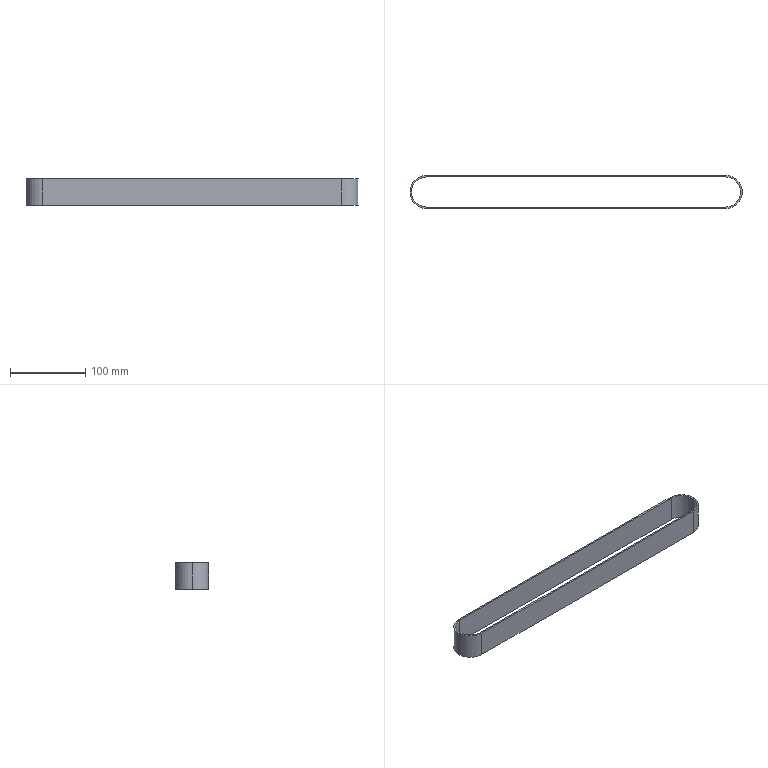Part | STEP file | Belt | 1 solid | 12 faces | box 442 x 44 x 35 mm | volume 64956 mm3 | cylinder 6 | plane 6 | commonest cylinder face diameters 40 x3 44 x3
STEP:
#1=CARTESIAN_POINT('',(0.,0.,0.));
#2=DIRECTION('',(0.,0.,1.));
#3=DIRECTION('',(1.,0.,0.));
#4=AXIS2_PLACEMENT_3D('',#1,#2,#3);
#5=CARTESIAN_POINT('',(-22.,0.,35.));
#6=VERTEX_POINT('',#5);
#7=CARTESIAN_POINT('',(0.,-22.,35.));
#8=VERTEX_POINT('',#7);
#9=CARTESIAN_POINT('',(0.,0.,35.));
#10=DIRECTION('',(0.,0.,1.));
#11=DIRECTION('',(-1.,0.,0.));
#12=AXIS2_PLACEMENT_3D('',#9,#10,#11);
#13=CIRCLE('',#12,22.);
#14=CARTESIAN_POINT('',(0.,0.,35.));
#15=DIRECTION('',(0.,0.,-1.));
#16=DIRECTION('',(-1.,0.,0.));
#17=AXIS2_PLACEMENT_3D('',#14,#15,#16);
#18=CYLINDRICAL_SURFACE('',#17,22.);
#19=CARTESIAN_POINT('',(6.283,0.));
#20=DIRECTION('',(-1.,0.));
#21=VECTOR('',#20,1.);
#22=LINE('',#19,#21);
#23=(GEOMETRIC_REPRESENTATION_CONTEXT(2)PARAMETRIC_REPRESENTATION_CONTEXT()REPRESENTATION_CONTEXT('',''));
#24=DEFINITIONAL_REPRESENTATION('',(#22),#23);
#25=PCURVE('',#18,#24);
#26=CARTESIAN_POINT('',(0.,0.,35.));
#27=DIRECTION('',(0.,0.,1.));
#28=DIRECTION('',(1.,0.,0.));
#29=AXIS2_PLACEMENT_3D('',#26,#27,#28);
#30=PLANE('',#29);
#31=CARTESIAN_POINT('',(0.,0.));
#32=DIRECTION('',(-1.,0.));
#33=AXIS2_PLACEMENT_2D('',#31,#32);
#34=CIRCLE('',#33,22.);
#35=(GEOMETRIC_REPRESENTATION_CONTEXT(2)PARAMETRIC_REPRESENTATION_CONTEXT()REPRESENTATION_CONTEXT('',''));
#36=DEFINITIONAL_REPRESENTATION('',(#34),#35);
#37=PCURVE('',#30,#36);
#38=SURFACE_CURVE('',#13,(#25,#37),.PCURVE_S1.);
#39=EDGE_CURVE('',#6,#8,#38,.T.);
#40=ORIENTED_EDGE('',*,*,#39,.F.);
#41=CARTESIAN_POINT('',(-22.,0.,0.));
#42=VERTEX_POINT('',#41);
#43=CARTESIAN_POINT('',(-22.,0.,35.));
#44=DIRECTION('',(0.,0.,-1.));
#45=VECTOR('',#44,1.);
#46=LINE('',#43,#45);
#47=CARTESIAN_POINT('',(6.283,0.));
#48=DIRECTION('',(0.,1.));
#49=VECTOR('',#48,1.);
#50=LINE('',#47,#49);
#51=(GEOMETRIC_REPRESENTATION_CONTEXT(2)PARAMETRIC_REPRESENTATION_CONTEXT()REPRESENTATION_CONTEXT('',''));
#52=DEFINITIONAL_REPRESENTATION('',(#50),#51);
#53=PCURVE('',#18,#52);
#54=CARTESIAN_POINT('',(0.,0.,35.));
#55=DIRECTION('',(0.,0.,-1.));
#56=DIRECTION('',(-1.,0.,0.));
#57=AXIS2_PLACEMENT_3D('',#54,#55,#56);
#58=CYLINDRICAL_SURFACE('',#57,22.);
#59=CARTESIAN_POINT('',(0.,0.));
#60=DIRECTION('',(0.,1.));
#61=VECTOR('',#60,1.);
#62=LINE('',#59,#61);
#63=(GEOMETRIC_REPRESENTATION_CONTEXT(2)PARAMETRIC_REPRESENTATION_CONTEXT()REPRESENTATION_CONTEXT('',''));
#64=DEFINITIONAL_REPRESENTATION('',(#62),#63);
#65=PCURVE('',#58,#64);
#66=SURFACE_CURVE('',#46,(#53,#65),.PCURVE_S1.);
#67=EDGE_CURVE('',#6,#42,#66,.T.);
#68=ORIENTED_EDGE('',*,*,#67,.T.);
#69=CARTESIAN_POINT('',(0.,-22.,0.));
#70=VERTEX_POINT('',#69);
#71=CARTESIAN_POINT('',(0.,0.,0.));
#72=DIRECTION('',(0.,0.,1.));
#73=DIRECTION('',(-1.,0.,0.));
#74=AXIS2_PLACEMENT_3D('',#71,#72,#73);
#75=CIRCLE('',#74,22.);
#76=CARTESIAN_POINT('',(6.283,35.));
#77=DIRECTION('',(-1.,0.));
#78=VECTOR('',#77,1.);
#79=LINE('',#76,#78);
#80=(GEOMETRIC_REPRESENTATION_CONTEXT(2)PARAMETRIC_REPRESENTATION_CONTEXT()REPRESENTATION_CONTEXT('',''));
#81=DEFINITIONAL_REPRESENTATION('',(#79),#80);
#82=PCURVE('',#18,#81);
#83=CARTESIAN_POINT('',(0.,0.,0.));
#84=DIRECTION('',(0.,0.,1.));
#85=DIRECTION('',(1.,0.,0.));
#86=AXIS2_PLACEMENT_3D('',#83,#84,#85);
#87=PLANE('',#86);
#88=CARTESIAN_POINT('',(0.,0.));
#89=DIRECTION('',(-1.,0.));
#90=AXIS2_PLACEMENT_2D('',#88,#89);
#91=CIRCLE('',#90,22.);
#92=(GEOMETRIC_REPRESENTATION_CONTEXT(2)PARAMETRIC_REPRESENTATION_CONTEXT()REPRESENTATION_CONTEXT('',''));
#93=DEFINITIONAL_REPRESENTATION('',(#91),#92);
#94=PCURVE('',#87,#93);
#95=SURFACE_CURVE('',#75,(#82,#94),.PCURVE_S1.);
#96=EDGE_CURVE('',#42,#70,#95,.T.);
#97=ORIENTED_EDGE('',*,*,#96,.T.);
#98=CARTESIAN_POINT('',(0.,-22.,35.));
#99=DIRECTION('',(0.,0.,1.));
#100=VECTOR('',#99,1.);
#101=LINE('',#98,#100);
#102=CARTESIAN_POINT('',(4.712,0.));
#103=DIRECTION('',(0.,-1.));
#104=VECTOR('',#103,1.);
#105=LINE('',#102,#104);
#106=(GEOMETRIC_REPRESENTATION_CONTEXT(2)PARAMETRIC_REPRESENTATION_CONTEXT()REPRESENTATION_CONTEXT('',''));
#107=DEFINITIONAL_REPRESENTATION('',(#105),#106);
#108=PCURVE('',#18,#107);
#109=CARTESIAN_POINT('',(0.,-22.,35.));
#110=DIRECTION('',(0.,1.,0.));
#111=DIRECTION('',(0.,0.,1.));
#112=AXIS2_PLACEMENT_3D('',#109,#110,#111);
#113=PLANE('',#112);
#114=CARTESIAN_POINT('',(0.,0.));
#115=DIRECTION('',(1.,0.));
#116=VECTOR('',#115,1.);
#117=LINE('',#114,#116);
#118=(GEOMETRIC_REPRESENTATION_CONTEXT(2)PARAMETRIC_REPRESENTATION_CONTEXT()REPRESENTATION_CONTEXT('',''));
#119=DEFINITIONAL_REPRESENTATION('',(#117),#118);
#120=PCURVE('',#113,#119);
#121=SURFACE_CURVE('',#101,(#108,#120),.PCURVE_S1.);
#122=EDGE_CURVE('',#70,#8,#121,.T.);
#123=ORIENTED_EDGE('',*,*,#122,.T.);
#124=EDGE_LOOP('',(#40,#68,#97,#123));
#125=FACE_BOUND('',#124,.T.);
#126=ADVANCED_FACE('',(#125),#18,.T.);
#127=CARTESIAN_POINT('',(0.,20.,35.));
#128=VERTEX_POINT('',#127);
#129=CARTESIAN_POINT('',(0.,20.,0.));
#130=VERTEX_POINT('',#129);
#131=CARTESIAN_POINT('',(0.,20.,35.));
#132=DIRECTION('',(0.,0.,-1.));
#133=VECTOR('',#132,1.);
#134=LINE('',#131,#133);
#135=CARTESIAN_POINT('',(0.,0.,35.));
#136=DIRECTION('',(0.,0.,-1.));
#137=DIRECTION('',(-1.,0.,0.));
#138=AXIS2_PLACEMENT_3D('',#135,#136,#137);
#139=CYLINDRICAL_SURFACE('',#138,20.);
#140=CARTESIAN_POINT('',(1.571,0.));
#141=DIRECTION('',(0.,1.));
#142=VECTOR('',#141,1.);
#143=LINE('',#140,#142);
#144=(GEOMETRIC_REPRESENTATION_CONTEXT(2)PARAMETRIC_REPRESENTATION_CONTEXT()REPRESENTATION_CONTEXT('',''));
#145=DEFINITIONAL_REPRESENTATION('',(#143),#144);
#146=PCURVE('',#139,#145);
#147=CARTESIAN_POINT('',(0.,20.,35.));
#148=DIRECTION('',(0.,-1.,0.));
#149=DIRECTION('',(0.,0.,-1.));
#150=AXIS2_PLACEMENT_3D('',#147,#148,#149);
#151=PLANE('',#150);
#152=CARTESIAN_POINT('',(0.,0.));
#153=DIRECTION('',(1.,0.));
#154=VECTOR('',#153,1.);
#155=LINE('',#152,#154);
#156=(GEOMETRIC_REPRESENTATION_CONTEXT(2)PARAMETRIC_REPRESENTATION_CONTEXT()REPRESENTATION_CONTEXT('',''));
#157=DEFINITIONAL_REPRESENTATION('',(#155),#156);
#158=PCURVE('',#151,#157);
#159=SURFACE_CURVE('',#134,(#146,#158),.PCURVE_S1.);
#160=EDGE_CURVE('',#128,#130,#159,.T.);
#161=ORIENTED_EDGE('',*,*,#160,.T.);
#162=CARTESIAN_POINT('',(-20.,0.,0.));
#163=VERTEX_POINT('',#162);
#164=CARTESIAN_POINT('',(0.,0.,0.));
#165=DIRECTION('',(0.,0.,-1.));
#166=DIRECTION('',(-1.,0.,0.));
#167=AXIS2_PLACEMENT_3D('',#164,#165,#166);
#168=CIRCLE('',#167,20.);
#169=CARTESIAN_POINT('',(0.,35.));
#170=DIRECTION('',(1.,0.));
#171=VECTOR('',#170,1.);
#172=LINE('',#169,#171);
#173=(GEOMETRIC_REPRESENTATION_CONTEXT(2)PARAMETRIC_REPRESENTATION_CONTEXT()REPRESENTATION_CONTEXT('',''));
#174=DEFINITIONAL_REPRESENTATION('',(#172),#173);
#175=PCURVE('',#139,#174);
#176=CARTESIAN_POINT('',(-20.,0.));
#177=CARTESIAN_POINT('',(-20.,34.641));
#178=CARTESIAN_POINT('',(10.,17.321));
#179=CARTESIAN_POINT('',(40.,0.));
#180=CARTESIAN_POINT('',(10.,-17.321));
#181=CARTESIAN_POINT('',(-20.,-34.641));
#182=CARTESIAN_POINT('',(-20.,0.));
#183=(BOUNDED_CURVE()B_SPLINE_CURVE(2,(#176,#177,#178,#179,#180,#181,#182),.UNSPECIFIED.,.T.,.F.)B_SPLINE_CURVE_WITH_KNOTS((1,2,2,2,2,1),(-2.094,0.,2.094,4.189,6.283,8.378),.UNSPECIFIED.)CURVE()GEOMETRIC_REPRESENTATION_ITEM()RATIONAL_B_SPLINE_CURVE((1.,0.5,1.,0.5,1.,0.5,1.))REPRESENTATION_ITEM(''));
#184=(GEOMETRIC_REPRESENTATION_CONTEXT(2)PARAMETRIC_REPRESENTATION_CONTEXT()REPRESENTATION_CONTEXT('',''));
#185=DEFINITIONAL_REPRESENTATION('',(#183),#184);
#186=PCURVE('',#87,#185);
#187=SURFACE_CURVE('',#168,(#175,#186),.PCURVE_S1.);
#188=EDGE_CURVE('',#163,#130,#187,.T.);
#189=ORIENTED_EDGE('',*,*,#188,.F.);
#190=CARTESIAN_POINT('',(-20.,0.,35.));
#191=VERTEX_POINT('',#190);
#192=CARTESIAN_POINT('',(-20.,0.,35.));
#193=DIRECTION('',(0.,0.,-1.));
#194=VECTOR('',#193,1.);
#195=LINE('',#192,#194);
#196=CARTESIAN_POINT('',(0.,0.));
#197=DIRECTION('',(0.,1.));
#198=VECTOR('',#197,1.);
#199=LINE('',#196,#198);
#200=(GEOMETRIC_REPRESENTATION_CONTEXT(2)PARAMETRIC_REPRESENTATION_CONTEXT()REPRESENTATION_CONTEXT('',''));
#201=DEFINITIONAL_REPRESENTATION('',(#199),#200);
#202=PCURVE('',#139,#201);
#203=CARTESIAN_POINT('',(0.,0.,35.));
#204=DIRECTION('',(0.,0.,-1.));
#205=DIRECTION('',(-1.,0.,0.));
#206=AXIS2_PLACEMENT_3D('',#203,#204,#205);
#207=CYLINDRICAL_SURFACE('',#206,20.);
#208=CARTESIAN_POINT('',(6.283,0.));
#209=DIRECTION('',(0.,1.));
#210=VECTOR('',#209,1.);
#211=LINE('',#208,#210);
#212=(GEOMETRIC_REPRESENTATION_CONTEXT(2)PARAMETRIC_REPRESENTATION_CONTEXT()REPRESENTATION_CONTEXT('',''));
#213=DEFINITIONAL_REPRESENTATION('',(#211),#212);
#214=PCURVE('',#207,#213);
#215=SURFACE_CURVE('',#195,(#202,#214),.PCURVE_S1.);
#216=EDGE_CURVE('',#191,#163,#215,.T.);
#217=ORIENTED_EDGE('',*,*,#216,.F.);
#218=CARTESIAN_POINT('',(0.,0.,35.));
#219=DIRECTION('',(0.,0.,-1.));
#220=DIRECTION('',(-1.,0.,0.));
#221=AXIS2_PLACEMENT_3D('',#218,#219,#220);
#222=CIRCLE('',#221,20.);
#223=CARTESIAN_POINT('',(0.,0.));
#224=DIRECTION('',(1.,0.));
#225=VECTOR('',#224,1.);
#226=LINE('',#223,#225);
#227=(GEOMETRIC_REPRESENTATION_CONTEXT(2)PARAMETRIC_REPRESENTATION_CONTEXT()REPRESENTATION_CONTEXT('',''));
#228=DEFINITIONAL_REPRESENTATION('',(#226),#227);
#229=PCURVE('',#139,#228);
#230=CARTESIAN_POINT('',(-20.,0.));
#231=CARTESIAN_POINT('',(-20.,34.641));
#232=CARTESIAN_POINT('',(10.,17.321));
#233=CARTESIAN_POINT('',(40.,0.));
#234=CARTESIAN_POINT('',(10.,-17.321));
#235=CARTESIAN_POINT('',(-20.,-34.641));
#236=CARTESIAN_POINT('',(-20.,0.));
#237=(BOUNDED_CURVE()B_SPLINE_CURVE(2,(#230,#231,#232,#233,#234,#235,#236),.UNSPECIFIED.,.T.,.F.)B_SPLINE_CURVE_WITH_KNOTS((1,2,2,2,2,1),(-2.094,0.,2.094,4.189,6.283,8.378),.UNSPECIFIED.)CURVE()GEOMETRIC_REPRESENTATION_ITEM()RATIONAL_B_SPLINE_CURVE((1.,0.5,1.,0.5,1.,0.5,1.))REPRESENTATION_ITEM(''));
#238=(GEOMETRIC_REPRESENTATION_CONTEXT(2)PARAMETRIC_REPRESENTATION_CONTEXT()REPRESENTATION_CONTEXT('',''));
#239=DEFINITIONAL_REPRESENTATION('',(#237),#238);
#240=PCURVE('',#30,#239);
#241=SURFACE_CURVE('',#222,(#229,#240),.PCURVE_S1.);
#242=EDGE_CURVE('',#191,#128,#241,.T.);
#243=ORIENTED_EDGE('',*,*,#242,.T.);
#244=EDGE_LOOP('',(#161,#189,#217,#243));
#245=FACE_BOUND('',#244,.F.);
#246=ADVANCED_FACE('',(#245),#139,.F.);
#247=CARTESIAN_POINT('',(398.,-22.,35.));
#248=VERTEX_POINT('',#247);
#249=CARTESIAN_POINT('',(398.,-22.,0.));
#250=VERTEX_POINT('',#249);
#251=CARTESIAN_POINT('',(398.,-22.,35.));
#252=DIRECTION('',(0.,0.,-1.));
#253=VECTOR('',#252,1.);
#254=LINE('',#251,#253);
#255=CARTESIAN_POINT('',(0.,398.));
#256=DIRECTION('',(-1.,0.));
#257=VECTOR('',#256,1.);
#258=LINE('',#255,#257);
#259=(GEOMETRIC_REPRESENTATION_CONTEXT(2)PARAMETRIC_REPRESENTATION_CONTEXT()REPRESENTATION_CONTEXT('',''));
#260=DEFINITIONAL_REPRESENTATION('',(#258),#259);
#261=PCURVE('',#113,#260);
#262=CARTESIAN_POINT('',(398.,0.,35.));
#263=DIRECTION('',(0.,0.,-1.));
#264=DIRECTION('',(-1.,0.,0.));
#265=AXIS2_PLACEMENT_3D('',#262,#263,#264);
#266=CYLINDRICAL_SURFACE('',#265,22.);
#267=CARTESIAN_POINT('',(4.712,0.));
#268=DIRECTION('',(0.,1.));
#269=VECTOR('',#268,1.);
#270=LINE('',#267,#269);
#271=(GEOMETRIC_REPRESENTATION_CONTEXT(2)PARAMETRIC_REPRESENTATION_CONTEXT()REPRESENTATION_CONTEXT('',''));
#272=DEFINITIONAL_REPRESENTATION('',(#270),#271);
#273=PCURVE('',#266,#272);
#274=SURFACE_CURVE('',#254,(#261,#273),.PCURVE_S1.);
#275=EDGE_CURVE('',#248,#250,#274,.T.);
#276=ORIENTED_EDGE('',*,*,#275,.F.);
#277=CARTESIAN_POINT('',(0.,-22.,35.));
#278=DIRECTION('',(1.,0.,0.));
#279=VECTOR('',#278,1.);
#280=LINE('',#277,#279);
#281=CARTESIAN_POINT('',(0.,0.));
#282=DIRECTION('',(0.,1.));
#283=VECTOR('',#282,1.);
#284=LINE('',#281,#283);
#285=(GEOMETRIC_REPRESENTATION_CONTEXT(2)PARAMETRIC_REPRESENTATION_CONTEXT()REPRESENTATION_CONTEXT('',''));
#286=DEFINITIONAL_REPRESENTATION('',(#284),#285);
#287=PCURVE('',#113,#286);
#288=CARTESIAN_POINT('',(0.,-22.));
#289=DIRECTION('',(1.,0.));
#290=VECTOR('',#289,1.);
#291=LINE('',#288,#290);
#292=(GEOMETRIC_REPRESENTATION_CONTEXT(2)PARAMETRIC_REPRESENTATION_CONTEXT()REPRESENTATION_CONTEXT('',''));
#293=DEFINITIONAL_REPRESENTATION('',(#291),#292);
#294=PCURVE('',#30,#293);
#295=SURFACE_CURVE('',#280,(#287,#294),.PCURVE_S1.);
#296=EDGE_CURVE('',#8,#248,#295,.T.);
#297=ORIENTED_EDGE('',*,*,#296,.F.);
#298=ORIENTED_EDGE('',*,*,#122,.F.);
#299=CARTESIAN_POINT('',(0.,-22.,0.));
#300=DIRECTION('',(-1.,0.,0.));
#301=VECTOR('',#300,1.);
#302=LINE('',#299,#301);
#303=CARTESIAN_POINT('',(-35.,0.));
#304=DIRECTION('',(0.,-1.));
#305=VECTOR('',#304,1.);
#306=LINE('',#303,#305);
#307=(GEOMETRIC_REPRESENTATION_CONTEXT(2)PARAMETRIC_REPRESENTATION_CONTEXT()REPRESENTATION_CONTEXT('',''));
#308=DEFINITIONAL_REPRESENTATION('',(#306),#307);
#309=PCURVE('',#113,#308);
#310=CARTESIAN_POINT('',(0.,-22.));
#311=DIRECTION('',(-1.,0.));
#312=VECTOR('',#311,1.);
#313=LINE('',#310,#312);
#314=(GEOMETRIC_REPRESENTATION_CONTEXT(2)PARAMETRIC_REPRESENTATION_CONTEXT()REPRESENTATION_CONTEXT('',''));
#315=DEFINITIONAL_REPRESENTATION('',(#313),#314);
#316=PCURVE('',#87,#315);
#317=SURFACE_CURVE('',#302,(#309,#316),.PCURVE_S1.);
#318=EDGE_CURVE('',#250,#70,#317,.T.);
#319=ORIENTED_EDGE('',*,*,#318,.F.);
#320=EDGE_LOOP('',(#276,#297,#298,#319));
#321=FACE_BOUND('',#320,.T.);
#322=ADVANCED_FACE('',(#321),#113,.F.);
#323=CARTESIAN_POINT('',(0.,-20.,0.));
#324=VERTEX_POINT('',#323);
#325=CARTESIAN_POINT('',(0.,0.,0.));
#326=DIRECTION('',(0.,0.,-1.));
#327=DIRECTION('',(-1.,0.,0.));
#328=AXIS2_PLACEMENT_3D('',#325,#326,#327);
#329=CIRCLE('',#328,20.);
#330=CARTESIAN_POINT('',(-20.,0.));
#331=CARTESIAN_POINT('',(-20.,34.641));
#332=CARTESIAN_POINT('',(10.,17.321));
#333=CARTESIAN_POINT('',(40.,0.));
#334=CARTESIAN_POINT('',(10.,-17.321));
#335=CARTESIAN_POINT('',(-20.,-34.641));
#336=CARTESIAN_POINT('',(-20.,0.));
#337=(BOUNDED_CURVE()B_SPLINE_CURVE(2,(#330,#331,#332,#333,#334,#335,#336),.UNSPECIFIED.,.T.,.F.)B_SPLINE_CURVE_WITH_KNOTS((1,2,2,2,2,1),(-2.094,0.,2.094,4.189,6.283,8.378),.UNSPECIFIED.)CURVE()GEOMETRIC_REPRESENTATION_ITEM()RATIONAL_B_SPLINE_CURVE((1.,0.5,1.,0.5,1.,0.5,1.))REPRESENTATION_ITEM(''));
#338=(GEOMETRIC_REPRESENTATION_CONTEXT(2)PARAMETRIC_REPRESENTATION_CONTEXT()REPRESENTATION_CONTEXT('',''));
#339=DEFINITIONAL_REPRESENTATION('',(#337),#338);
#340=PCURVE('',#87,#339);
#341=CARTESIAN_POINT('',(0.,35.));
#342=DIRECTION('',(1.,0.));
#343=VECTOR('',#342,1.);
#344=LINE('',#341,#343);
#345=(GEOMETRIC_REPRESENTATION_CONTEXT(2)PARAMETRIC_REPRESENTATION_CONTEXT()REPRESENTATION_CONTEXT('',''));
#346=DEFINITIONAL_REPRESENTATION('',(#344),#345);
#347=PCURVE('',#207,#346);
#348=SURFACE_CURVE('',#329,(#340,#347),.PCURVE_S1.);
#349=EDGE_CURVE('',#324,#163,#348,.T.);
#350=ORIENTED_EDGE('',*,*,#349,.F.);
#351=CARTESIAN_POINT('',(398.,-20.,0.));
#352=VERTEX_POINT('',#351);
#353=CARTESIAN_POINT('',(0.,-20.,0.));
#354=DIRECTION('',(-1.,0.,0.));
#355=VECTOR('',#354,1.);
#356=LINE('',#353,#355);
#357=CARTESIAN_POINT('',(0.,-20.));
#358=DIRECTION('',(-1.,0.));
#359=VECTOR('',#358,1.);
#360=LINE('',#357,#359);
#361=(GEOMETRIC_REPRESENTATION_CONTEXT(2)PARAMETRIC_REPRESENTATION_CONTEXT()REPRESENTATION_CONTEXT('',''));
#362=DEFINITIONAL_REPRESENTATION('',(#360),#361);
#363=PCURVE('',#87,#362);
#364=CARTESIAN_POINT('',(0.,-20.,35.));
#365=DIRECTION('',(0.,1.,0.));
#366=DIRECTION('',(0.,0.,1.));
#367=AXIS2_PLACEMENT_3D('',#364,#365,#366);
#368=PLANE('',#367);
#369=CARTESIAN_POINT('',(-35.,0.));
#370=DIRECTION('',(0.,-1.));
#371=VECTOR('',#370,1.);
#372=LINE('',#369,#371);
#373=(GEOMETRIC_REPRESENTATION_CONTEXT(2)PARAMETRIC_REPRESENTATION_CONTEXT()REPRESENTATION_CONTEXT('',''));
#374=DEFINITIONAL_REPRESENTATION('',(#372),#373);
#375=PCURVE('',#368,#374);
#376=SURFACE_CURVE('',#356,(#363,#375),.PCURVE_S1.);
#377=EDGE_CURVE('',#352,#324,#376,.T.);
#378=ORIENTED_EDGE('',*,*,#377,.F.);
#379=CARTESIAN_POINT('',(398.,20.,0.));
#380=VERTEX_POINT('',#379);
#381=CARTESIAN_POINT('',(398.,0.,0.));
#382=DIRECTION('',(0.,0.,-1.));
#383=DIRECTION('',(-1.,0.,0.));
#384=AXIS2_PLACEMENT_3D('',#381,#382,#383);
#385=CIRCLE('',#384,20.);
#386=CARTESIAN_POINT('',(378.,0.));
#387=CARTESIAN_POINT('',(378.,34.641));
#388=CARTESIAN_POINT('',(408.,17.321));
#389=CARTESIAN_POINT('',(438.,0.));
#390=CARTESIAN_POINT('',(408.,-17.321));
#391=CARTESIAN_POINT('',(378.,-34.641));
#392=CARTESIAN_POINT('',(378.,0.));
#393=(BOUNDED_CURVE()B_SPLINE_CURVE(2,(#386,#387,#388,#389,#390,#391,#392),.UNSPECIFIED.,.T.,.F.)B_SPLINE_CURVE_WITH_KNOTS((1,2,2,2,2,1),(-2.094,0.,2.094,4.189,6.283,8.378),.UNSPECIFIED.)CURVE()GEOMETRIC_REPRESENTATION_ITEM()RATIONAL_B_SPLINE_CURVE((1.,0.5,1.,0.5,1.,0.5,1.))REPRESENTATION_ITEM(''));
#394=(GEOMETRIC_REPRESENTATION_CONTEXT(2)PARAMETRIC_REPRESENTATION_CONTEXT()REPRESENTATION_CONTEXT('',''));
#395=DEFINITIONAL_REPRESENTATION('',(#393),#394);
#396=PCURVE('',#87,#395);
#397=CARTESIAN_POINT('',(398.,0.,35.));
#398=DIRECTION('',(0.,0.,-1.));
#399=DIRECTION('',(-1.,0.,0.));
#400=AXIS2_PLACEMENT_3D('',#397,#398,#399);
#401=CYLINDRICAL_SURFACE('',#400,20.);
#402=CARTESIAN_POINT('',(0.,35.));
#403=DIRECTION('',(1.,0.));
#404=VECTOR('',#403,1.);
#405=LINE('',#402,#404);
#406=(GEOMETRIC_REPRESENTATION_CONTEXT(2)PARAMETRIC_REPRESENTATION_CONTEXT()REPRESENTATION_CONTEXT('',''));
#407=DEFINITIONAL_REPRESENTATION('',(#405),#406);
#408=PCURVE('',#401,#407);
#409=SURFACE_CURVE('',#385,(#396,#408),.PCURVE_S1.);
#410=EDGE_CURVE('',#380,#352,#409,.T.);
#411=ORIENTED_EDGE('',*,*,#410,.F.);
#412=CARTESIAN_POINT('',(0.,20.,0.));
#413=DIRECTION('',(1.,0.,0.));
#414=VECTOR('',#413,1.);
#415=LINE('',#412,#414);
#416=CARTESIAN_POINT('',(0.,20.));
#417=DIRECTION('',(1.,0.));
#418=VECTOR('',#417,1.);
#419=LINE('',#416,#418);
#420=(GEOMETRIC_REPRESENTATION_CONTEXT(2)PARAMETRIC_REPRESENTATION_CONTEXT()REPRESENTATION_CONTEXT('',''));
#421=DEFINITIONAL_REPRESENTATION('',(#419),#420);
#422=PCURVE('',#87,#421);
#423=CARTESIAN_POINT('',(35.,0.));
#424=DIRECTION('',(0.,1.));
#425=VECTOR('',#424,1.);
#426=LINE('',#423,#425);
#427=(GEOMETRIC_REPRESENTATION_CONTEXT(2)PARAMETRIC_REPRESENTATION_CONTEXT()REPRESENTATION_CONTEXT('',''));
#428=DEFINITIONAL_REPRESENTATION('',(#426),#427);
#429=PCURVE('',#151,#428);
#430=SURFACE_CURVE('',#415,(#422,#429),.PCURVE_S1.);
#431=EDGE_CURVE('',#130,#380,#430,.T.);
#432=ORIENTED_EDGE('',*,*,#431,.F.);
#433=ORIENTED_EDGE('',*,*,#188,.F.);
#434=EDGE_LOOP('',(#350,#378,#411,#432,#433));
#435=FACE_BOUND('',#434,.T.);
#436=CARTESIAN_POINT('',(398.,22.,0.));
#437=VERTEX_POINT('',#436);
#438=CARTESIAN_POINT('',(0.,22.,0.));
#439=VERTEX_POINT('',#438);
#440=CARTESIAN_POINT('',(0.,22.,0.));
#441=DIRECTION('',(-1.,0.,0.));
#442=VECTOR('',#441,1.);
#443=LINE('',#440,#442);
#444=CARTESIAN_POINT('',(0.,22.));
#445=DIRECTION('',(-1.,0.));
#446=VECTOR('',#445,1.);
#447=LINE('',#444,#446);
#448=(GEOMETRIC_REPRESENTATION_CONTEXT(2)PARAMETRIC_REPRESENTATION_CONTEXT()REPRESENTATION_CONTEXT('',''));
#449=DEFINITIONAL_REPRESENTATION('',(#447),#448);
#450=PCURVE('',#87,#449);
#451=CARTESIAN_POINT('',(0.,22.,35.));
#452=DIRECTION('',(0.,-1.,0.));
#453=DIRECTION('',(0.,0.,-1.));
#454=AXIS2_PLACEMENT_3D('',#451,#452,#453);
#455=PLANE('',#454);
#456=CARTESIAN_POINT('',(35.,0.));
#457=DIRECTION('',(0.,-1.));
#458=VECTOR('',#457,1.);
#459=LINE('',#456,#458);
#460=(GEOMETRIC_REPRESENTATION_CONTEXT(2)PARAMETRIC_REPRESENTATION_CONTEXT()REPRESENTATION_CONTEXT('',''));
#461=DEFINITIONAL_REPRESENTATION('',(#459),#460);
#462=PCURVE('',#455,#461);
#463=SURFACE_CURVE('',#443,(#450,#462),.PCURVE_S1.);
#464=EDGE_CURVE('',#437,#439,#463,.T.);
#465=ORIENTED_EDGE('',*,*,#464,.F.);
#466=CARTESIAN_POINT('',(398.,0.,0.));
#467=DIRECTION('',(0.,0.,1.));
#468=DIRECTION('',(-1.,0.,0.));
#469=AXIS2_PLACEMENT_3D('',#466,#467,#468);
#470=CIRCLE('',#469,22.);
#471=CARTESIAN_POINT('',(398.,0.));
#472=DIRECTION('',(-1.,0.));
#473=AXIS2_PLACEMENT_2D('',#471,#472);
#474=CIRCLE('',#473,22.);
#475=(GEOMETRIC_REPRESENTATION_CONTEXT(2)PARAMETRIC_REPRESENTATION_CONTEXT()REPRESENTATION_CONTEXT('',''));
#476=DEFINITIONAL_REPRESENTATION('',(#474),#475);
#477=PCURVE('',#87,#476);
#478=CARTESIAN_POINT('',(6.283,35.));
#479=DIRECTION('',(-1.,0.));
#480=VECTOR('',#479,1.);
#481=LINE('',#478,#480);
#482=(GEOMETRIC_REPRESENTATION_CONTEXT(2)PARAMETRIC_REPRESENTATION_CONTEXT()REPRESENTATION_CONTEXT('',''));
#483=DEFINITIONAL_REPRESENTATION('',(#481),#482);
#484=PCURVE('',#266,#483);
#485=SURFACE_CURVE('',#470,(#477,#484),.PCURVE_S1.);
#486=EDGE_CURVE('',#250,#437,#485,.T.);
#487=ORIENTED_EDGE('',*,*,#486,.F.);
#488=ORIENTED_EDGE('',*,*,#318,.T.);
#489=ORIENTED_EDGE('',*,*,#96,.F.);
#490=CARTESIAN_POINT('',(0.,0.,0.));
#491=DIRECTION('',(0.,0.,1.));
#492=DIRECTION('',(-1.,0.,0.));
#493=AXIS2_PLACEMENT_3D('',#490,#491,#492);
#494=CIRCLE('',#493,22.);
#495=CARTESIAN_POINT('',(0.,0.));
#496=DIRECTION('',(-1.,0.));
#497=AXIS2_PLACEMENT_2D('',#495,#496);
#498=CIRCLE('',#497,22.);
#499=(GEOMETRIC_REPRESENTATION_CONTEXT(2)PARAMETRIC_REPRESENTATION_CONTEXT()REPRESENTATION_CONTEXT('',''));
#500=DEFINITIONAL_REPRESENTATION('',(#498),#499);
#501=PCURVE('',#87,#500);
#502=CARTESIAN_POINT('',(6.283,35.));
#503=DIRECTION('',(-1.,0.));
#504=VECTOR('',#503,1.);
#505=LINE('',#502,#504);
#506=(GEOMETRIC_REPRESENTATION_CONTEXT(2)PARAMETRIC_REPRESENTATION_CONTEXT()REPRESENTATION_CONTEXT('',''));
#507=DEFINITIONAL_REPRESENTATION('',(#505),#506);
#508=PCURVE('',#58,#507);
#509=SURFACE_CURVE('',#494,(#501,#508),.PCURVE_S1.);
#510=EDGE_CURVE('',#439,#42,#509,.T.);
#511=ORIENTED_EDGE('',*,*,#510,.F.);
#512=EDGE_LOOP('',(#465,#487,#488,#489,#511));
#513=FACE_BOUND('',#512,.T.);
#514=ADVANCED_FACE('',(#435,#513),#87,.F.);
#515=CARTESIAN_POINT('',(398.,22.,35.));
#516=VERTEX_POINT('',#515);
#517=CARTESIAN_POINT('',(398.,0.,35.));
#518=DIRECTION('',(0.,0.,-1.));
#519=DIRECTION('',(-1.,0.,0.));
#520=AXIS2_PLACEMENT_3D('',#517,#518,#519);
#521=CIRCLE('',#520,22.);
#522=CARTESIAN_POINT('',(0.,0.));
#523=DIRECTION('',(1.,0.));
#524=VECTOR('',#523,1.);
#525=LINE('',#522,#524);
#526=(GEOMETRIC_REPRESENTATION_CONTEXT(2)PARAMETRIC_REPRESENTATION_CONTEXT()REPRESENTATION_CONTEXT('',''));
#527=DEFINITIONAL_REPRESENTATION('',(#525),#526);
#528=PCURVE('',#266,#527);
#529=CARTESIAN_POINT('',(376.,0.));
#530=CARTESIAN_POINT('',(376.,38.105));
#531=CARTESIAN_POINT('',(409.,19.053));
#532=CARTESIAN_POINT('',(442.,0.));
#533=CARTESIAN_POINT('',(409.,-19.053));
#534=CARTESIAN_POINT('',(376.,-38.105));
#535=CARTESIAN_POINT('',(376.,0.));
#536=(BOUNDED_CURVE()B_SPLINE_CURVE(2,(#529,#530,#531,#532,#533,#534,#535),.UNSPECIFIED.,.T.,.F.)B_SPLINE_CURVE_WITH_KNOTS((1,2,2,2,2,1),(-2.094,0.,2.094,4.189,6.283,8.378),.UNSPECIFIED.)CURVE()GEOMETRIC_REPRESENTATION_ITEM()RATIONAL_B_SPLINE_CURVE((1.,0.5,1.,0.5,1.,0.5,1.))REPRESENTATION_ITEM(''));
#537=(GEOMETRIC_REPRESENTATION_CONTEXT(2)PARAMETRIC_REPRESENTATION_CONTEXT()REPRESENTATION_CONTEXT('',''));
#538=DEFINITIONAL_REPRESENTATION('',(#536),#537);
#539=PCURVE('',#30,#538);
#540=SURFACE_CURVE('',#521,(#528,#539),.PCURVE_S1.);
#541=EDGE_CURVE('',#516,#248,#540,.T.);
#542=ORIENTED_EDGE('',*,*,#541,.T.);
#543=ORIENTED_EDGE('',*,*,#275,.T.);
#544=ORIENTED_EDGE('',*,*,#486,.T.);
#545=CARTESIAN_POINT('',(398.,22.,35.));
#546=DIRECTION('',(0.,0.,1.));
#547=VECTOR('',#546,1.);
#548=LINE('',#545,#547);
#549=CARTESIAN_POINT('',(1.571,0.));
#550=DIRECTION('',(0.,-1.));
#551=VECTOR('',#550,1.);
#552=LINE('',#549,#551);
#553=(GEOMETRIC_REPRESENTATION_CONTEXT(2)PARAMETRIC_REPRESENTATION_CONTEXT()REPRESENTATION_CONTEXT('',''));
#554=DEFINITIONAL_REPRESENTATION('',(#552),#553);
#555=PCURVE('',#266,#554);
#556=CARTESIAN_POINT('',(0.,398.));
#557=DIRECTION('',(-1.,0.));
#558=VECTOR('',#557,1.);
#559=LINE('',#556,#558);
#560=(GEOMETRIC_REPRESENTATION_CONTEXT(2)PARAMETRIC_REPRESENTATION_CONTEXT()REPRESENTATION_CONTEXT('',''));
#561=DEFINITIONAL_REPRESENTATION('',(#559),#560);
#562=PCURVE('',#455,#561);
#563=SURFACE_CURVE('',#548,(#555,#562),.PCURVE_S1.);
#564=EDGE_CURVE('',#437,#516,#563,.T.);
#565=ORIENTED_EDGE('',*,*,#564,.T.);
#566=EDGE_LOOP('',(#542,#543,#544,#565));
#567=FACE_BOUND('',#566,.T.);
#568=ADVANCED_FACE('',(#567),#266,.T.);
#569=CARTESIAN_POINT('',(398.,20.,35.));
#570=VERTEX_POINT('',#569);
#571=CARTESIAN_POINT('',(0.,20.,35.));
#572=DIRECTION('',(1.,0.,0.));
#573=VECTOR('',#572,1.);
#574=LINE('',#571,#573);
#575=CARTESIAN_POINT('',(0.,20.));
#576=DIRECTION('',(1.,0.));
#577=VECTOR('',#576,1.);
#578=LINE('',#575,#577);
#579=(GEOMETRIC_REPRESENTATION_CONTEXT(2)PARAMETRIC_REPRESENTATION_CONTEXT()REPRESENTATION_CONTEXT('',''));
#580=DEFINITIONAL_REPRESENTATION('',(#578),#579);
#581=PCURVE('',#30,#580);
#582=CARTESIAN_POINT('',(0.,0.));
#583=DIRECTION('',(0.,1.));
#584=VECTOR('',#583,1.);
#585=LINE('',#582,#584);
#586=(GEOMETRIC_REPRESENTATION_CONTEXT(2)PARAMETRIC_REPRESENTATION_CONTEXT()REPRESENTATION_CONTEXT('',''));
#587=DEFINITIONAL_REPRESENTATION('',(#585),#586);
#588=PCURVE('',#151,#587);
#589=SURFACE_CURVE('',#574,(#581,#588),.PCURVE_S1.);
#590=EDGE_CURVE('',#128,#570,#589,.T.);
#591=ORIENTED_EDGE('',*,*,#590,.T.);
#592=CARTESIAN_POINT('',(398.,-20.,35.));
#593=VERTEX_POINT('',#592);
#594=CARTESIAN_POINT('',(398.,0.,35.));
#595=DIRECTION('',(0.,0.,-1.));
#596=DIRECTION('',(-1.,0.,0.));
#597=AXIS2_PLACEMENT_3D('',#594,#595,#596);
#598=CIRCLE('',#597,20.);
#599=CARTESIAN_POINT('',(378.,0.));
#600=CARTESIAN_POINT('',(378.,34.641));
#601=CARTESIAN_POINT('',(408.,17.321));
#602=CARTESIAN_POINT('',(438.,0.));
#603=CARTESIAN_POINT('',(408.,-17.321));
#604=CARTESIAN_POINT('',(378.,-34.641));
#605=CARTESIAN_POINT('',(378.,0.));
#606=(BOUNDED_CURVE()B_SPLINE_CURVE(2,(#599,#600,#601,#602,#603,#604,#605),.UNSPECIFIED.,.T.,.F.)B_SPLINE_CURVE_WITH_KNOTS((1,2,2,2,2,1),(-2.094,0.,2.094,4.189,6.283,8.378),.UNSPECIFIED.)CURVE()GEOMETRIC_REPRESENTATION_ITEM()RATIONAL_B_SPLINE_CURVE((1.,0.5,1.,0.5,1.,0.5,1.))REPRESENTATION_ITEM(''));
#607=(GEOMETRIC_REPRESENTATION_CONTEXT(2)PARAMETRIC_REPRESENTATION_CONTEXT()REPRESENTATION_CONTEXT('',''));
#608=DEFINITIONAL_REPRESENTATION('',(#606),#607);
#609=PCURVE('',#30,#608);
#610=CARTESIAN_POINT('',(0.,0.));
#611=DIRECTION('',(1.,0.));
#612=VECTOR('',#611,1.);
#613=LINE('',#610,#612);
#614=(GEOMETRIC_REPRESENTATION_CONTEXT(2)PARAMETRIC_REPRESENTATION_CONTEXT()REPRESENTATION_CONTEXT('',''));
#615=DEFINITIONAL_REPRESENTATION('',(#613),#614);
#616=PCURVE('',#401,#615);
#617=SURFACE_CURVE('',#598,(#609,#616),.PCURVE_S1.);
#618=EDGE_CURVE('',#570,#593,#617,.T.);
#619=ORIENTED_EDGE('',*,*,#618,.T.);
#620=CARTESIAN_POINT('',(0.,-20.,35.));
#621=VERTEX_POINT('',#620);
#622=CARTESIAN_POINT('',(0.,-20.,35.));
#623=DIRECTION('',(-1.,0.,0.));
#624=VECTOR('',#623,1.);
#625=LINE('',#622,#624);
#626=CARTESIAN_POINT('',(0.,-20.));
#627=DIRECTION('',(-1.,0.));
#628=VECTOR('',#627,1.);
#629=LINE('',#626,#628);
#630=(GEOMETRIC_REPRESENTATION_CONTEXT(2)PARAMETRIC_REPRESENTATION_CONTEXT()REPRESENTATION_CONTEXT('',''));
#631=DEFINITIONAL_REPRESENTATION('',(#629),#630);
#632=PCURVE('',#30,#631);
#633=CARTESIAN_POINT('',(0.,0.));
#634=DIRECTION('',(0.,-1.));
#635=VECTOR('',#634,1.);
#636=LINE('',#633,#635);
#637=(GEOMETRIC_REPRESENTATION_CONTEXT(2)PARAMETRIC_REPRESENTATION_CONTEXT()REPRESENTATION_CONTEXT('',''));
#638=DEFINITIONAL_REPRESENTATION('',(#636),#637);
#639=PCURVE('',#368,#638);
#640=SURFACE_CURVE('',#625,(#632,#639),.PCURVE_S1.);
#641=EDGE_CURVE('',#593,#621,#640,.T.);
#642=ORIENTED_EDGE('',*,*,#641,.T.);
#643=CARTESIAN_POINT('',(0.,0.,35.));
#644=DIRECTION('',(0.,0.,-1.));
#645=DIRECTION('',(-1.,0.,0.));
#646=AXIS2_PLACEMENT_3D('',#643,#644,#645);
#647=CIRCLE('',#646,20.);
#648=CARTESIAN_POINT('',(-20.,0.));
#649=CARTESIAN_POINT('',(-20.,34.641));
#650=CARTESIAN_POINT('',(10.,17.321));
#651=CARTESIAN_POINT('',(40.,0.));
#652=CARTESIAN_POINT('',(10.,-17.321));
#653=CARTESIAN_POINT('',(-20.,-34.641));
#654=CARTESIAN_POINT('',(-20.,0.));
#655=(BOUNDED_CURVE()B_SPLINE_CURVE(2,(#648,#649,#650,#651,#652,#653,#654),.UNSPECIFIED.,.T.,.F.)B_SPLINE_CURVE_WITH_KNOTS((1,2,2,2,2,1),(-2.094,0.,2.094,4.189,6.283,8.378),.UNSPECIFIED.)CURVE()GEOMETRIC_REPRESENTATION_ITEM()RATIONAL_B_SPLINE_CURVE((1.,0.5,1.,0.5,1.,0.5,1.))REPRESENTATION_ITEM(''));
#656=(GEOMETRIC_REPRESENTATION_CONTEXT(2)PARAMETRIC_REPRESENTATION_CONTEXT()REPRESENTATION_CONTEXT('',''));
#657=DEFINITIONAL_REPRESENTATION('',(#655),#656);
#658=PCURVE('',#30,#657);
#659=CARTESIAN_POINT('',(0.,0.));
#660=DIRECTION('',(1.,0.));
#661=VECTOR('',#660,1.);
#662=LINE('',#659,#661);
#663=(GEOMETRIC_REPRESENTATION_CONTEXT(2)PARAMETRIC_REPRESENTATION_CONTEXT()REPRESENTATION_CONTEXT('',''));
#664=DEFINITIONAL_REPRESENTATION('',(#662),#663);
#665=PCURVE('',#207,#664);
#666=SURFACE_CURVE('',#647,(#658,#665),.PCURVE_S1.);
#667=EDGE_CURVE('',#621,#191,#666,.T.);
#668=ORIENTED_EDGE('',*,*,#667,.T.);
#669=ORIENTED_EDGE('',*,*,#242,.T.);
#670=EDGE_LOOP('',(#591,#619,#642,#668,#669));
#671=FACE_BOUND('',#670,.T.);
#672=ORIENTED_EDGE('',*,*,#541,.F.);
#673=CARTESIAN_POINT('',(0.,22.,35.));
#674=VERTEX_POINT('',#673);
#675=CARTESIAN_POINT('',(0.,22.,35.));
#676=DIRECTION('',(-1.,0.,0.));
#677=VECTOR('',#676,1.);
#678=LINE('',#675,#677);
#679=CARTESIAN_POINT('',(0.,22.));
#680=DIRECTION('',(-1.,0.));
#681=VECTOR('',#680,1.);
#682=LINE('',#679,#681);
#683=(GEOMETRIC_REPRESENTATION_CONTEXT(2)PARAMETRIC_REPRESENTATION_CONTEXT()REPRESENTATION_CONTEXT('',''));
#684=DEFINITIONAL_REPRESENTATION('',(#682),#683);
#685=PCURVE('',#30,#684);
#686=CARTESIAN_POINT('',(0.,0.));
#687=DIRECTION('',(0.,-1.));
#688=VECTOR('',#687,1.);
#689=LINE('',#686,#688);
#690=(GEOMETRIC_REPRESENTATION_CONTEXT(2)PARAMETRIC_REPRESENTATION_CONTEXT()REPRESENTATION_CONTEXT('',''));
#691=DEFINITIONAL_REPRESENTATION('',(#689),#690);
#692=PCURVE('',#455,#691);
#693=SURFACE_CURVE('',#678,(#685,#692),.PCURVE_S1.);
#694=EDGE_CURVE('',#516,#674,#693,.T.);
#695=ORIENTED_EDGE('',*,*,#694,.T.);
#696=CARTESIAN_POINT('',(0.,0.,35.));
#697=DIRECTION('',(0.,0.,1.));
#698=DIRECTION('',(-1.,0.,0.));
#699=AXIS2_PLACEMENT_3D('',#696,#697,#698);
#700=CIRCLE('',#699,22.);
#701=CARTESIAN_POINT('',(0.,0.));
#702=DIRECTION('',(-1.,0.));
#703=AXIS2_PLACEMENT_2D('',#701,#702);
#704=CIRCLE('',#703,22.);
#705=(GEOMETRIC_REPRESENTATION_CONTEXT(2)PARAMETRIC_REPRESENTATION_CONTEXT()REPRESENTATION_CONTEXT('',''));
#706=DEFINITIONAL_REPRESENTATION('',(#704),#705);
#707=PCURVE('',#30,#706);
#708=CARTESIAN_POINT('',(6.283,0.));
#709=DIRECTION('',(-1.,0.));
#710=VECTOR('',#709,1.);
#711=LINE('',#708,#710);
#712=(GEOMETRIC_REPRESENTATION_CONTEXT(2)PARAMETRIC_REPRESENTATION_CONTEXT()REPRESENTATION_CONTEXT('',''));
#713=DEFINITIONAL_REPRESENTATION('',(#711),#712);
#714=PCURVE('',#58,#713);
#715=SURFACE_CURVE('',#700,(#707,#714),.PCURVE_S1.);
#716=EDGE_CURVE('',#674,#6,#715,.T.);
#717=ORIENTED_EDGE('',*,*,#716,.T.);
#718=ORIENTED_EDGE('',*,*,#39,.T.);
#719=ORIENTED_EDGE('',*,*,#296,.T.);
#720=EDGE_LOOP('',(#672,#695,#717,#718,#719));
#721=FACE_BOUND('',#720,.T.);
#722=ADVANCED_FACE('',(#671,#721),#30,.T.);
#723=ORIENTED_EDGE('',*,*,#67,.F.);
#724=ORIENTED_EDGE('',*,*,#716,.F.);
#725=CARTESIAN_POINT('',(0.,22.,35.));
#726=DIRECTION('',(0.,0.,-1.));
#727=VECTOR('',#726,1.);
#728=LINE('',#725,#727);
#729=CARTESIAN_POINT('',(1.571,0.));
#730=DIRECTION('',(0.,1.));
#731=VECTOR('',#730,1.);
#732=LINE('',#729,#731);
#733=(GEOMETRIC_REPRESENTATION_CONTEXT(2)PARAMETRIC_REPRESENTATION_CONTEXT()REPRESENTATION_CONTEXT('',''));
#734=DEFINITIONAL_REPRESENTATION('',(#732),#733);
#735=PCURVE('',#58,#734);
#736=CARTESIAN_POINT('',(0.,0.));
#737=DIRECTION('',(1.,0.));
#738=VECTOR('',#737,1.);
#739=LINE('',#736,#738);
#740=(GEOMETRIC_REPRESENTATION_CONTEXT(2)PARAMETRIC_REPRESENTATION_CONTEXT()REPRESENTATION_CONTEXT('',''));
#741=DEFINITIONAL_REPRESENTATION('',(#739),#740);
#742=PCURVE('',#455,#741);
#743=SURFACE_CURVE('',#728,(#735,#742),.PCURVE_S1.);
#744=EDGE_CURVE('',#674,#439,#743,.T.);
#745=ORIENTED_EDGE('',*,*,#744,.T.);
#746=ORIENTED_EDGE('',*,*,#510,.T.);
#747=EDGE_LOOP('',(#723,#724,#745,#746));
#748=FACE_BOUND('',#747,.T.);
#749=ADVANCED_FACE('',(#748),#58,.T.);
#750=ORIENTED_EDGE('',*,*,#349,.F.);
#751=CARTESIAN_POINT('',(0.,-20.,35.));
#752=DIRECTION('',(0.,0.,1.));
#753=VECTOR('',#752,1.);
#754=LINE('',#751,#753);
#755=CARTESIAN_POINT('',(4.712,0.));
#756=DIRECTION('',(0.,-1.));
#757=VECTOR('',#756,1.);
#758=LINE('',#755,#757);
#759=(GEOMETRIC_REPRESENTATION_CONTEXT(2)PARAMETRIC_REPRESENTATION_CONTEXT()REPRESENTATION_CONTEXT('',''));
#760=DEFINITIONAL_REPRESENTATION('',(#758),#759);
#761=PCURVE('',#207,#760);
#762=CARTESIAN_POINT('',(0.,0.));
#763=DIRECTION('',(1.,0.));
#764=VECTOR('',#763,1.);
#765=LINE('',#762,#764);
#766=(GEOMETRIC_REPRESENTATION_CONTEXT(2)PARAMETRIC_REPRESENTATION_CONTEXT()REPRESENTATION_CONTEXT('',''));
#767=DEFINITIONAL_REPRESENTATION('',(#765),#766);
#768=PCURVE('',#368,#767);
#769=SURFACE_CURVE('',#754,(#761,#768),.PCURVE_S1.);
#770=EDGE_CURVE('',#324,#621,#769,.T.);
#771=ORIENTED_EDGE('',*,*,#770,.T.);
#772=ORIENTED_EDGE('',*,*,#667,.T.);
#773=ORIENTED_EDGE('',*,*,#216,.T.);
#774=EDGE_LOOP('',(#750,#771,#772,#773));
#775=FACE_BOUND('',#774,.F.);
#776=ADVANCED_FACE('',(#775),#207,.F.);
#777=ORIENTED_EDGE('',*,*,#641,.F.);
#778=CARTESIAN_POINT('',(398.,-20.,35.));
#779=DIRECTION('',(0.,0.,-1.));
#780=VECTOR('',#779,1.);
#781=LINE('',#778,#780);
#782=CARTESIAN_POINT('',(0.,398.));
#783=DIRECTION('',(-1.,0.));
#784=VECTOR('',#783,1.);
#785=LINE('',#782,#784);
#786=(GEOMETRIC_REPRESENTATION_CONTEXT(2)PARAMETRIC_REPRESENTATION_CONTEXT()REPRESENTATION_CONTEXT('',''));
#787=DEFINITIONAL_REPRESENTATION('',(#785),#786);
#788=PCURVE('',#368,#787);
#789=CARTESIAN_POINT('',(4.712,0.));
#790=DIRECTION('',(0.,1.));
#791=VECTOR('',#790,1.);
#792=LINE('',#789,#791);
#793=(GEOMETRIC_REPRESENTATION_CONTEXT(2)PARAMETRIC_REPRESENTATION_CONTEXT()REPRESENTATION_CONTEXT('',''));
#794=DEFINITIONAL_REPRESENTATION('',(#792),#793);
#795=PCURVE('',#401,#794);
#796=SURFACE_CURVE('',#781,(#788,#795),.PCURVE_S1.);
#797=EDGE_CURVE('',#593,#352,#796,.T.);
#798=ORIENTED_EDGE('',*,*,#797,.T.);
#799=ORIENTED_EDGE('',*,*,#377,.T.);
#800=ORIENTED_EDGE('',*,*,#770,.T.);
#801=EDGE_LOOP('',(#777,#798,#799,#800));
#802=FACE_BOUND('',#801,.T.);
#803=ADVANCED_FACE('',(#802),#368,.T.);
#804=ORIENTED_EDGE('',*,*,#410,.F.);
#805=CARTESIAN_POINT('',(398.,20.,35.));
#806=DIRECTION('',(0.,0.,1.));
#807=VECTOR('',#806,1.);
#808=LINE('',#805,#807);
#809=CARTESIAN_POINT('',(1.571,0.));
#810=DIRECTION('',(0.,-1.));
#811=VECTOR('',#810,1.);
#812=LINE('',#809,#811);
#813=(GEOMETRIC_REPRESENTATION_CONTEXT(2)PARAMETRIC_REPRESENTATION_CONTEXT()REPRESENTATION_CONTEXT('',''));
#814=DEFINITIONAL_REPRESENTATION('',(#812),#813);
#815=PCURVE('',#401,#814);
#816=CARTESIAN_POINT('',(0.,398.));
#817=DIRECTION('',(-1.,0.));
#818=VECTOR('',#817,1.);
#819=LINE('',#816,#818);
#820=(GEOMETRIC_REPRESENTATION_CONTEXT(2)PARAMETRIC_REPRESENTATION_CONTEXT()REPRESENTATION_CONTEXT('',''));
#821=DEFINITIONAL_REPRESENTATION('',(#819),#820);
#822=PCURVE('',#151,#821);
#823=SURFACE_CURVE('',#808,(#815,#822),.PCURVE_S1.);
#824=EDGE_CURVE('',#380,#570,#823,.T.);
#825=ORIENTED_EDGE('',*,*,#824,.T.);
#826=ORIENTED_EDGE('',*,*,#618,.T.);
#827=ORIENTED_EDGE('',*,*,#797,.T.);
#828=EDGE_LOOP('',(#804,#825,#826,#827));
#829=FACE_BOUND('',#828,.F.);
#830=ADVANCED_FACE('',(#829),#401,.F.);
#831=ORIENTED_EDGE('',*,*,#590,.F.);
#832=ORIENTED_EDGE('',*,*,#160,.T.);
#833=ORIENTED_EDGE('',*,*,#431,.T.);
#834=ORIENTED_EDGE('',*,*,#824,.T.);
#835=EDGE_LOOP('',(#831,#832,#833,#834));
#836=FACE_BOUND('',#835,.T.);
#837=ADVANCED_FACE('',(#836),#151,.T.);
#838=ORIENTED_EDGE('',*,*,#744,.F.);
#839=ORIENTED_EDGE('',*,*,#694,.F.);
#840=ORIENTED_EDGE('',*,*,#564,.F.);
#841=ORIENTED_EDGE('',*,*,#464,.T.);
#842=EDGE_LOOP('',(#838,#839,#840,#841));
#843=FACE_BOUND('',#842,.T.);
#844=ADVANCED_FACE('',(#843),#455,.F.);
#845=CLOSED_SHELL('',(#126,#246,#322,#514,#568,#722,#749,#776,#803,#830,#837,#844));
#846=MANIFOLD_SOLID_BREP('',#845);
#847=(LENGTH_UNIT()NAMED_UNIT(*)SI_UNIT(.MILLI.,.METRE.));
#848=UNCERTAINTY_MEASURE_WITH_UNIT(LENGTH_MEASURE(0.0000001),#847,'','');
#849=(NAMED_UNIT(*)PLANE_ANGLE_UNIT()SI_UNIT($,.RADIAN.));
#850=(NAMED_UNIT(*)SI_UNIT($,.STERADIAN.)SOLID_ANGLE_UNIT());
#851=(GEOMETRIC_REPRESENTATION_CONTEXT(3)GLOBAL_UNCERTAINTY_ASSIGNED_CONTEXT((#848))GLOBAL_UNIT_ASSIGNED_CONTEXT((#847,#849,#850))REPRESENTATION_CONTEXT('',''));
#852=ADVANCED_BREP_SHAPE_REPRESENTATION('',(#4,#846),#851);